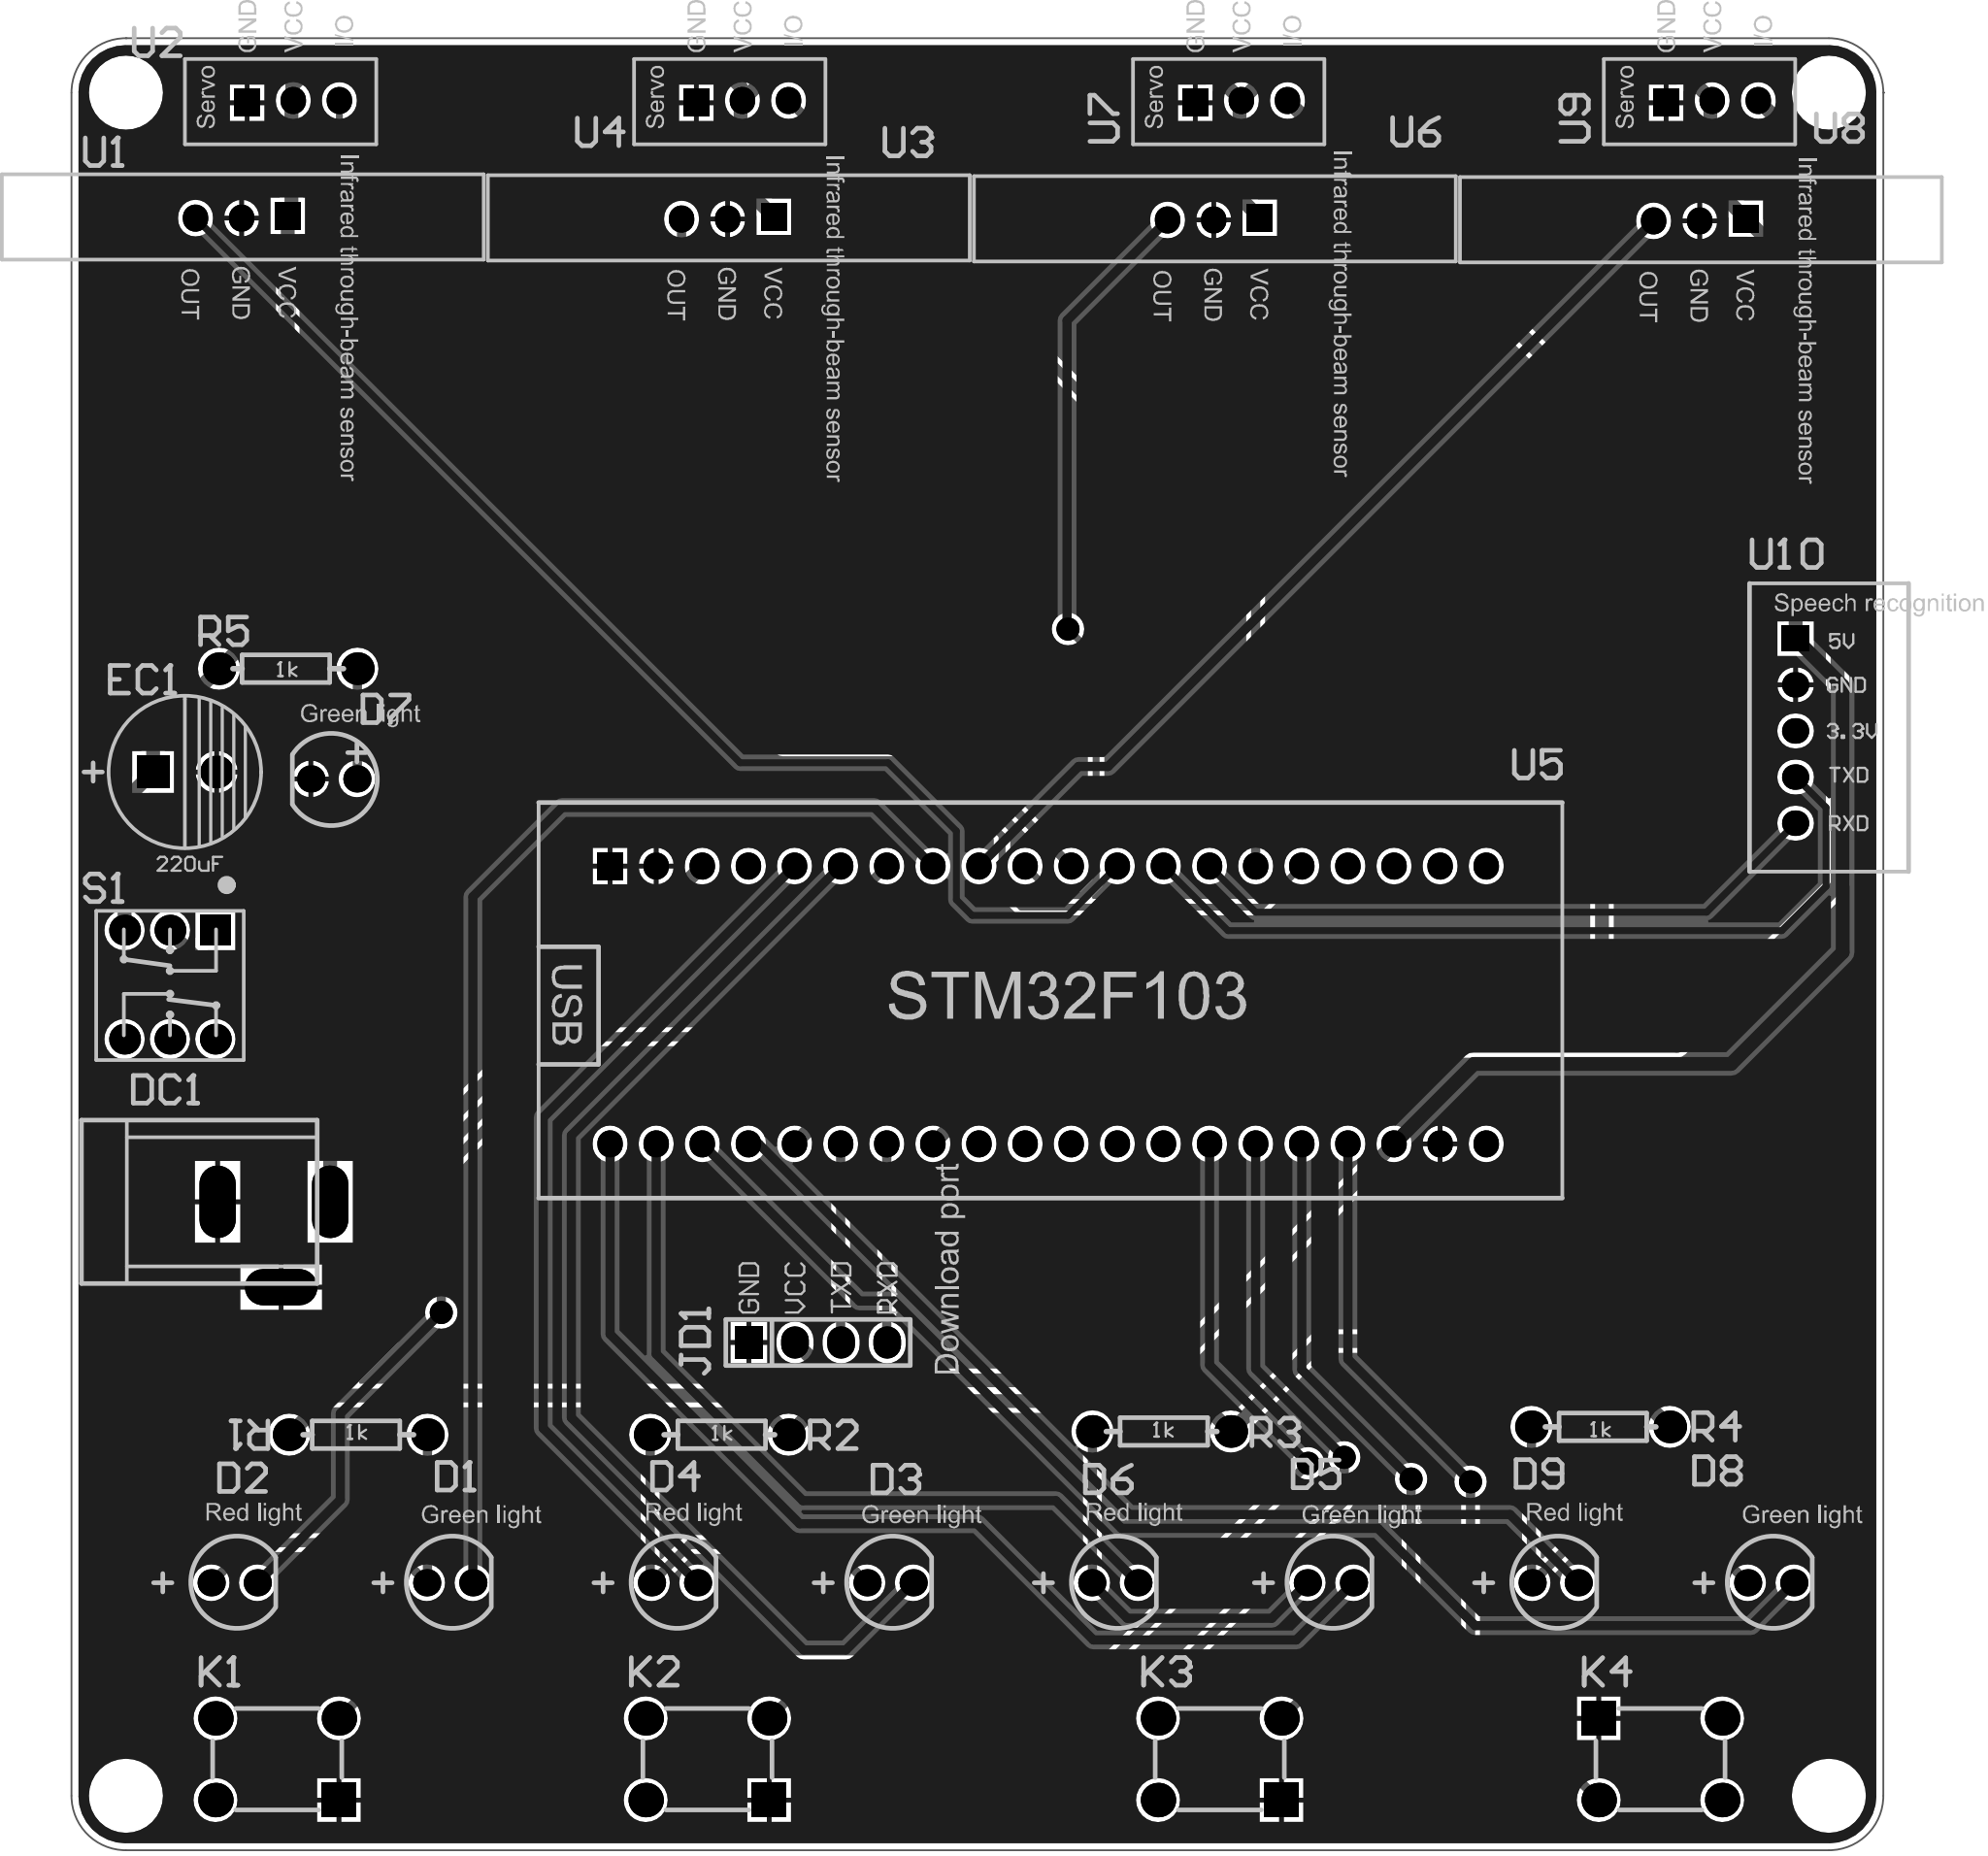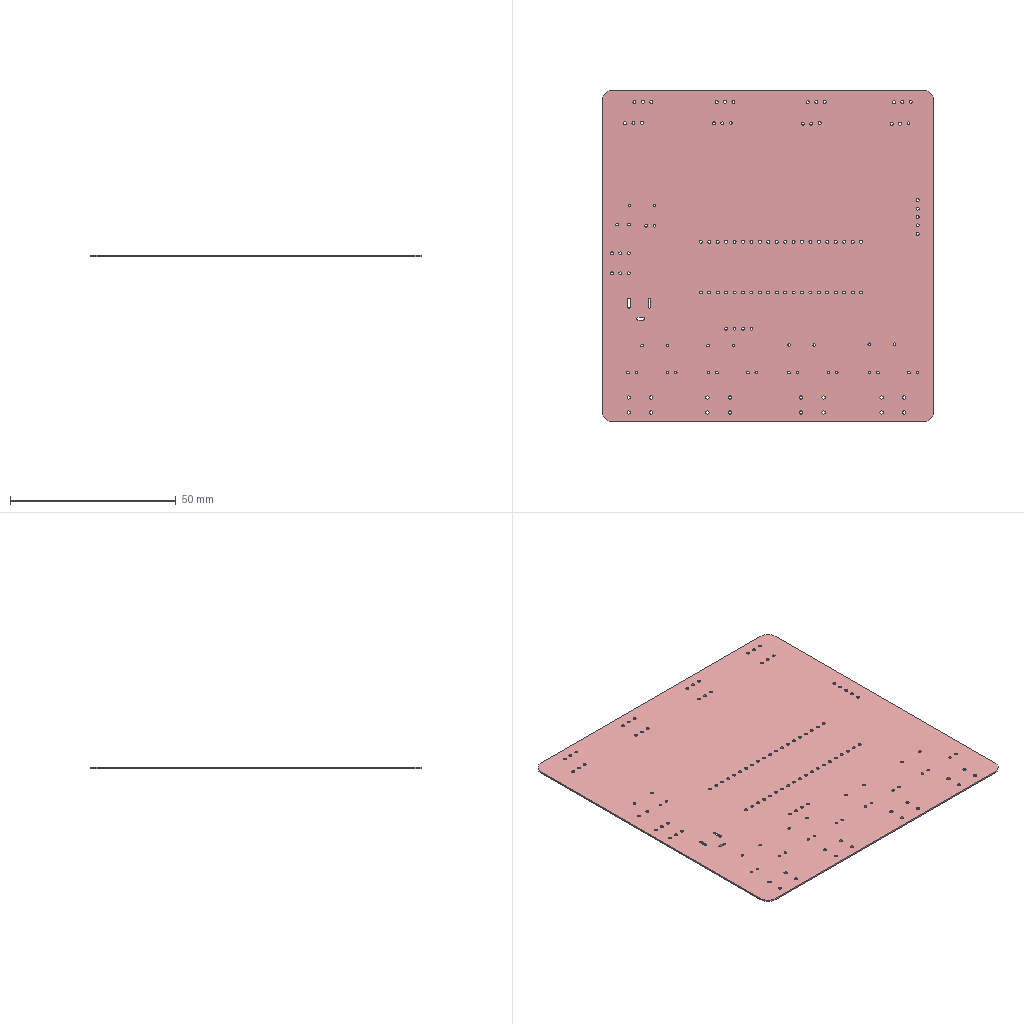Circuit board layout | Altium Designer | box 99.8 x 99.8 x 0.5 mm
Layer stack:
# Altium Designer layer stack of  (unit mm; dielectric type: 0 none, 1 core, 2 prepreg, 3 surface material)
index,name,kind,layer,copper_thickness_mm,dielectric_type,dielectric_thickness_mm,dielectric_material,dielectric_constant
0,Top Paste Mask Layer,other,,,,,,
1,Top Silkscreen Layer,other,,,,,,
2,Top Solder Mask Layer,dielectric,,,3,0.0356,FR-4,4.8
3,Top Layer,copper,Top Layer,0.0356,,,,
4,Substrate1,dielectric,,,3,0.32,FR-4,4.8
5,Bottom Layer,copper,Bottom Layer,0.0356,,,,
6,Bottom Solder Mask Layer,dielectric,,,3,0.0356,FR-4,4.8
7,Bottom Silkscreen Layer,other,,,,,,
8,Bottom Paste Mask Layer,other,,,,,,
# drill layer pairs: low layer,high layer
drill_pair,Top Layer,Bottom Layer
Part placement:
Designator,Comment,Layer,Footprint,Center-X(mm),Center-Y(mm),Rotation
JD1,Download port,TopLayer,下载口,126.924,123.495,180
U2,SG90,TopLayer,SG90,98.019,191.833,90
U1,JS,TopLayer,JS,95.174,185.483,270
D1,LED,TopLayer,LED5-GRE,106.64,110.261,0
D7,LED,TopLayer,LED5-GRE,100.254,154.534,180
K3,BUTTOM,TopLayer,DIP-6X6X5,149.051,100.544,180
K2,BUTTOM,TopLayer,DIP-6X6X5,120.831,100.544,180
K1,BUTTOM,TopLayer,DIP-6X6X5,97.133,100.544,180
R3,1k,TopLayer,AXIAL0.3-1k,145.847,118.593,0
R2,1K,TopLayer,AXIAL0.3-1k,121.488,118.415,0
R1,1k,TopLayer,AXIAL0.3-1k,101.6,118.415,180
EC1,220uF,TopLayer,DIP-EC3.5X8X11.5,92.047,154.915,0
DC1,DC_Socket,TopLayer,DC-005,96.951,128.892,180
S1,KFT DIP-8X8,TopLayer,KFT_DIP-8X8,91.226,143.202,270
D2,LED,TopLayer,LED5-RED,94.767,110.261,0
D3,LED,TopLayer,LED5-GRE,130.893,110.261,0
D4,LED,TopLayer,LED5-RED,119.021,110.261,0
D5,LED,TopLayer,LED5-GRE,155.147,110.261,0
D6,LED,TopLayer,LED5-RED,143.274,110.261,0
D8,LED,TopLayer,LED5-GRE,179.4,110.261,0
D9,LED,TopLayer,LED5-RED,167.528,110.261,0
K4,BUTTOM,TopLayer,DIP-6X6X5,173.326,100.544,0
R4,1k,TopLayer,AXIAL0.3-1k,170.028,118.847,0
R5,1k,TopLayer,AXIAL0.3-1k,97.739,160.604,180
U3,JS,TopLayer,JS,121.945,185.433,270
U4,SG90,TopLayer,SG90,122.758,191.833,90
U5,STM32F103,TopLayer,STM32F103,139.598,142.083,270
U6,JS,TopLayer,JS,148.717,185.382,270
U7,SG90,TopLayer,SG90,150.241,191.833,90
U8,JS,TopLayer,JS,175.489,185.331,270
U9,SG90,TopLayer,SG90,176.174,191.833,90
U10,SNR8016,TopLayer,SNR8016,180.772,157.175,0
Pad and via stacks:
# Altium Designer via and pad stacks of  (unit mm). Each distinct definition once, with the count of objects using it.
# via: kind,start_layer,end_layer,hole_mm,diameter_mm,mode(0 simple;1 top-mid-bottom;2 full stack),diameter_per_layer,count,example_net
# pad: kind,layer,hole_mm,hole_type(0 round;1 square;2 slot),plating,top_size,top_shape(1 round;2 rect;3 octagon;9 rounded rect),mid_size,bottom_size,mode,footprint,size_per_layer,count,example
pad,Multi-Layer,0.8128,0,plated,1.524x1.778,2,1.524x1.778,1.524x1.778,0,\u00CF\u00C2\u00D4\u00D8\u00BF\u00DA,,1,JD1.1
pad,Multi-Layer,0.8128,0,plated,1.524x1.778,1,1.524x1.778,1.524x1.778,0,\u00CF\u00C2\u00D4\u00D8\u00BF\u00DA,,3,JD1.4
pad,Multi-Layer,0.9,0,plated,1.4x1.5,2,1.4x1.5,1.4x1.5,0,SG90,,4,U2.1
pad,Multi-Layer,0.9,0,plated,1.4x1.5,1,1.4x1.5,1.4x1.5,0,SG90,,8,U2.2
pad,Multi-Layer,0.9,0,plated,1.4x1.5,1,1.4x1.5,1.4x1.5,0,JS,,8,U1.3
pad,Multi-Layer,0.9,0,plated,1.4x1.5,2,1.4x1.5,1.4x1.5,0,JS,,4,U1.1
pad,Multi-Layer,0.762,0,plated,1.5x1.5,1,1.5x1.5,1.5x1.5,0,LED5-GRE,,10,D1.A
pad,Multi-Layer,1,0,plated,1.9x1.9,1,1.9x1.9,1.9x1.9,0,DIP-6X6X5,,12,K3.4
pad,Multi-Layer,1,0,plated,1.9x1.9,2,1.9x1.9,1.9x1.9,0,DIP-6X6X5,,4,K3.1
pad,Multi-Layer,0.8,0,plated,1.8x1.8,1,1.8x1.8,1.8x1.8,0,AXIAL0.3-1k,,10,R3.1
pad,Multi-Layer,0.9,0,plated,1.8x1.8,1,1.8x1.8,1.8x1.8,0,DIP-EC3.5X8X11.5,,1,EC1.2
pad,Multi-Layer,0.9,0,plated,1.8x1.8,2,1.8x1.8,1.8x1.8,0,DIP-EC3.5X8X11.5,,1,EC1.1
pad,Multi-Layer,0.8,2,plated,2x4,1,2x4,2x4,0,DC-005,,2,DC1.1
pad,Multi-Layer,0.8,2,plated,4x2,1,4x2,4x2,0,DC-005,,1,DC1.3
pad,Multi-Layer,0.9,0,plated,1.7x1.7,1,1.7x1.7,1.7x1.7,0,KFT DIP-8X8,,5,S1.6
pad,Multi-Layer,0.9,0,plated,1.7x1.7,2,1.7x1.7,1.7x1.7,0,KFT DIP-8X8,,1,S1.1
pad,Multi-Layer,0.762,0,plated,1.5x1.5,1,1.5x1.5,1.5x1.5,0,LED5-RED,,8,D2.A
pad,Multi-Layer,0.9,0,plated,1.4x1.5,1,1.4x1.5,1.4x1.5,0,STM32F103,,39,U5.20
pad,Multi-Layer,0.9,0,plated,1.4x1.5,2,1.4x1.5,1.4x1.5,0,STM32F103,,1,U5.1
pad,Multi-Layer,0.9,0,plated,1.4x1.5,1,1.4x1.5,1.4x1.5,0,SNR8016,,4,U10.4
pad,Multi-Layer,0.9,0,plated,1.4x1.5,2,1.4x1.5,1.4x1.5,0,SNR8016,,1,U10.1
via,Top Layer,Bottom Layer,0.7112,1.27,0,,6,PA6
Copper pours:
name,layer,net,type(0 solid;1 hatched;2 none)
Bottom Layer-GND,Bottom Layer,GND,0
Top Layer-GND,Top Layer,GND,0
Design rules, without the lines most boards share:
# Altium Designer design rules of  (exported by Altium Designer, unit mm)
# columns: name | kind | enabled | priority | scope1 | scope2 | descriptor | typed fields (field=value)
ComponentClearance_1 | 24 | enabled | 1 | All | All | Component Clearance Constraint ( Horizontal Gap = 10mil, Vertical Gap = 10mil ) (All),(All)  | gap=0.254
Clearance | 0 | enabled | 1 | All | All | Clearance Constraint (Gap=10mil) (All),(All) | gap=0.254
Clearance_1 | 63 | enabled | 1 | All | All | Board Clearance Constraint (Gap=0mil) (All) |
ComponentClearance | 52 | enabled | 1 | All | All | Hole To Hole Clearance (Gap=10mil) (All),(All) | gap=0.254
Width | 2 | enabled | 1 | All | All | Width Constraint (Min=10mil) (Max=40mil) (Preferred=20mil) (All) |
DiffPairsRouting | 51 | enabled | 1 | All | All | Differential Pairs Uncoupled Length using the Gap Constraints (Min=10mil) (Max=10mil) (Prefered=10mil)  and Width Constraints (Min=99999mil) (Max=0mil) (Prefered=0mil) (All) |
RoutingVias | 11 | enabled | 1 | All | All | Routing Via (MinHoleWidth=28mil) (MaxHoleWidth=28mil) (PreferredHoleWidth=28mil) (MinWidth=50mil) (MaxWidth=50mil) (PreferedWidth=50mil) (All) | via_min_hole=0.7112 via_max_hole=0.7112 via_preferred_diameter=1.27 via_preferred_hole=0.7112
PlaneConnect | 6 | enabled | 1 | All | All | Power Plane Connect Rule(Relief Connect )(Expansion=20mil) (Conductor Width=10mil) (Air Gap=10mil) (Entries=4) (All) | relief_conductor_width=0.254 relief_entries=4 relief_expansion=0.508
PolygonConnect | 20 | enabled | 1 | All | All | Polygon Connect Rule(Relief Connect )(Conductor Width=10mil) (Relief Angle=90 Angle) (Entries=4) (Air Gap Width=10mil) (All),(All) | connect_style(0=relief,1=direct,2=none)=0 relief_conductor_width=0.254 relief_entries=4
PasteMaskExpansion | 14 | enabled | 1 | All | All | Paste Mask Expansion (Expansion =0mil) (All) | expansion=0
SolderMaskExpansion | 13 | enabled | 1 | All | All | Solder Mask Expansion (Expansion =4mil) (All) | expansion=0.1016